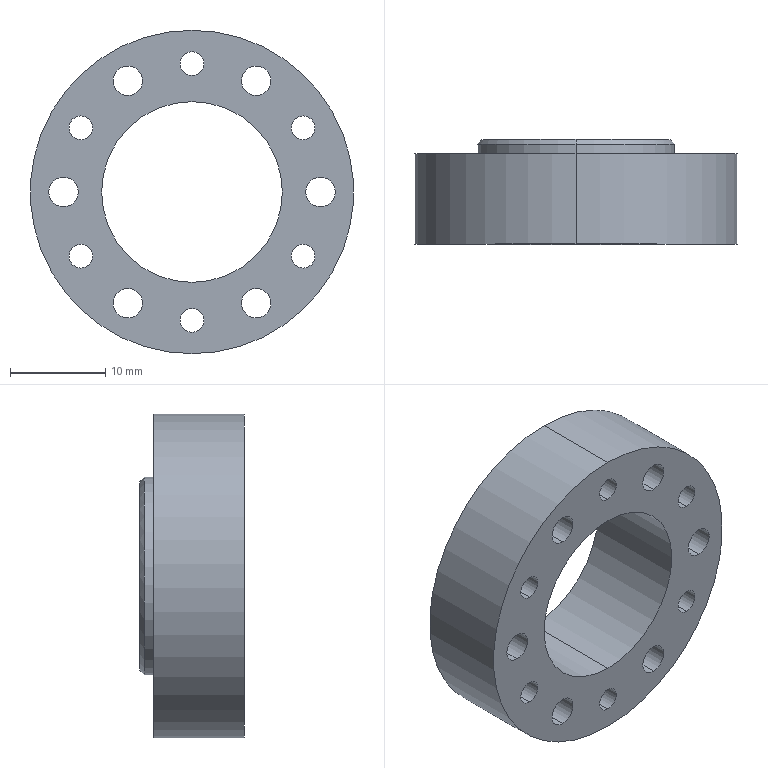Part | SolidWorks | features ICE 2, Chamfer 1, Extrusion 1, HoleWzd 1 | 1 solid | 65 faces | box 34 x 11 x 34 mm | volume 4612 mm3 | cylinder 42 | cone 14 | plane 9 | commonest cylinder face diameters 2.5 x12 3.1 x12 6 x12 19 x2 20.8 x2 34 x2